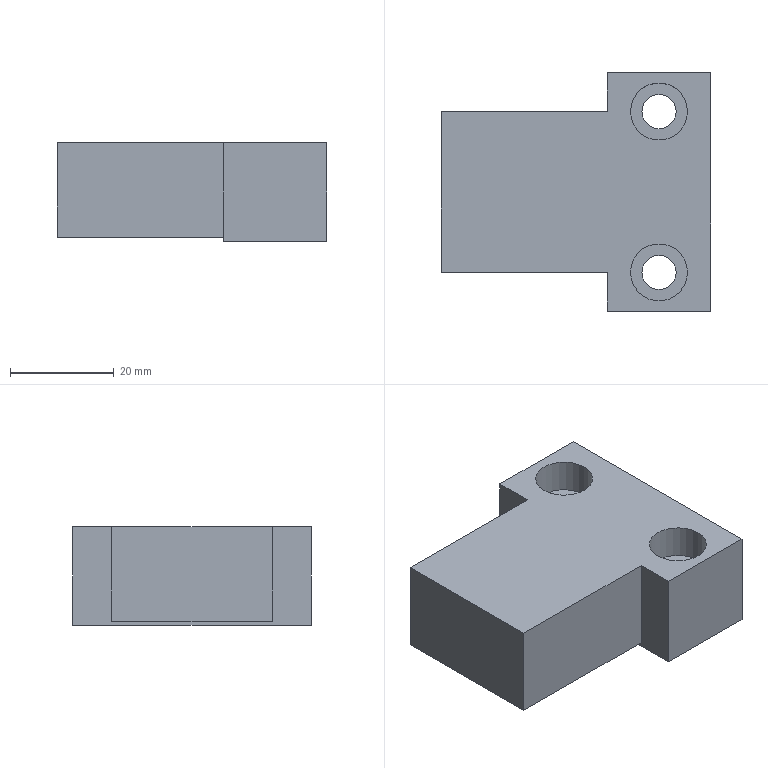Part | STEP file | solid 237 | 1 solid | 16 faces | box 52 x 46 x 19 mm | volume 33444 mm3 | plane 12 | cylinder 4 | commonest cylinder face diameters 6.6 x2 11 x2